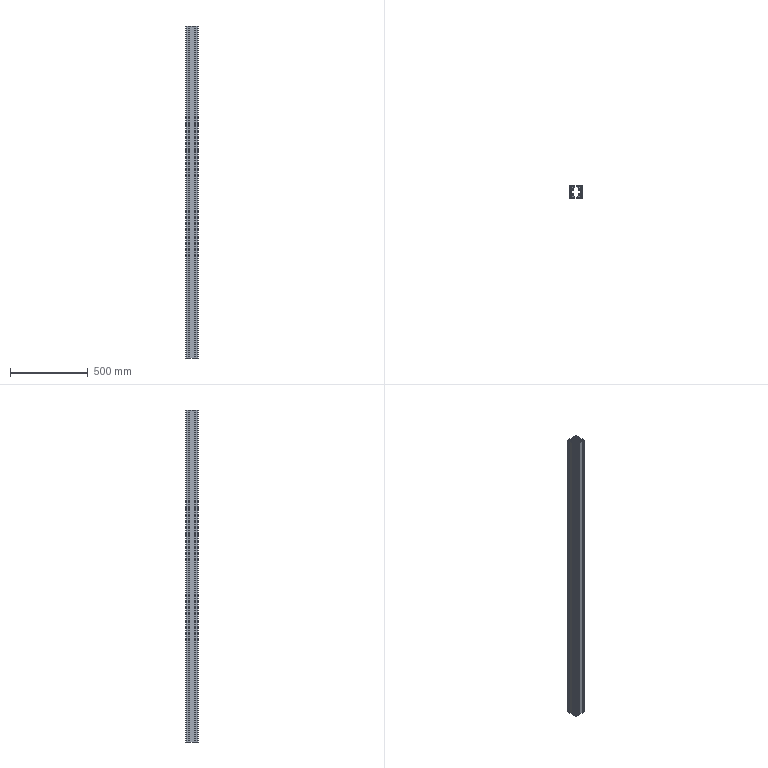Part | NX | 1 solid | 156 faces | box 80 x 80 x 2140 mm | volume 3749285 mm3 | plane 122 | cylinder 34 | commonest cylinder face diameters 2 x16 6.8 x8 11.8 x6 5.64 x4